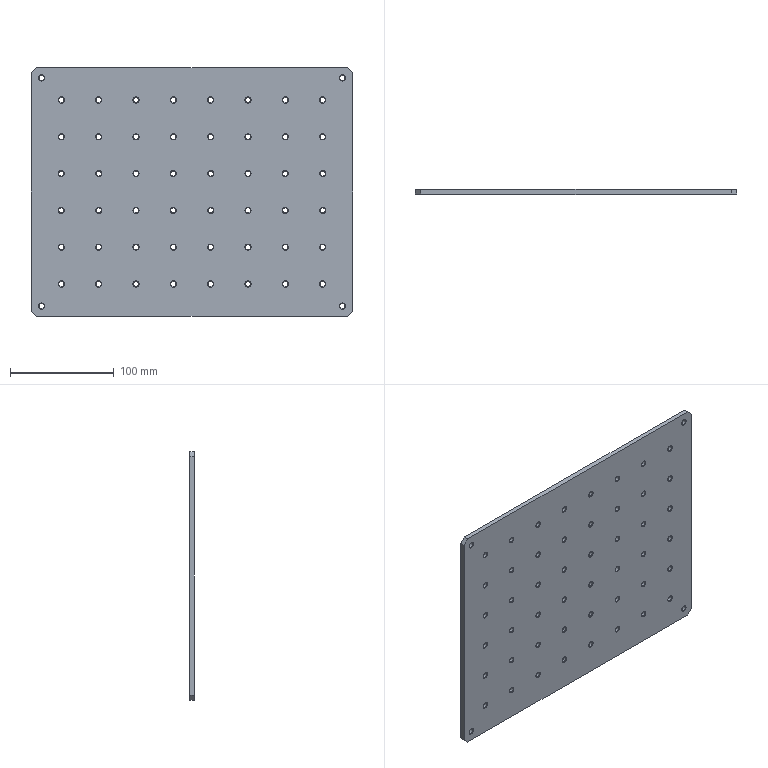Part | STEP file | Three-part square aluminium plate (2R8, 6R5) | 1 solid | 1090 faces | box 310 x 4.5 x 240 mm | volume 298192 mm3 | plane 490 | cylinder 392 | cone 208 | commonest cylinder face diameters 1.5 x288 5 x104